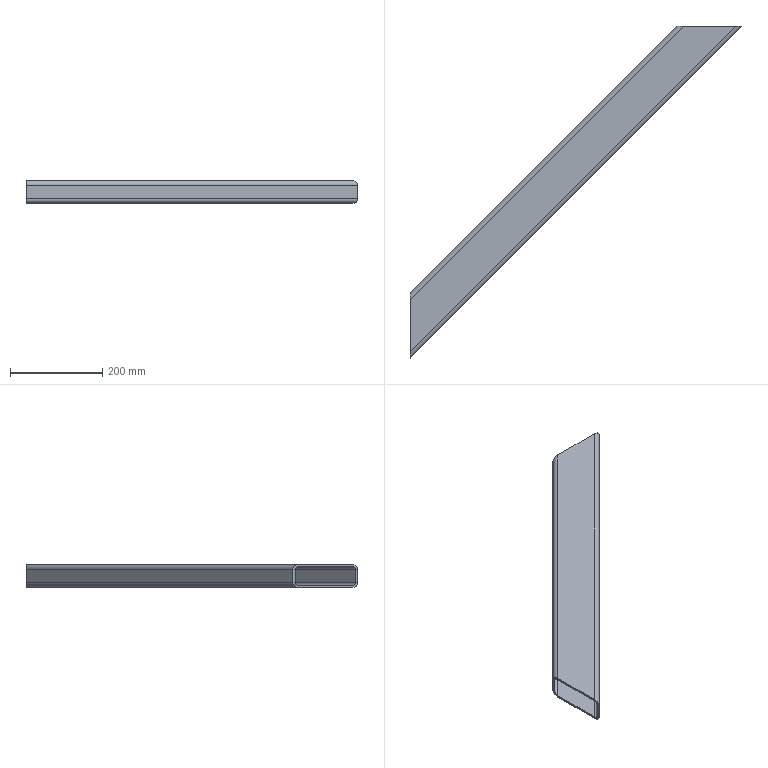Part | STEP file | Diagonal Brace矩形管-100×50-45度_Default<As Machined> | 1 solid | 18 faces | box 721.249 x 721.249 x 50 mm | volume 994577 mm3 | plane 10 | cylinder 8 | commonest cylinder face diameters 12 x4 20 x4